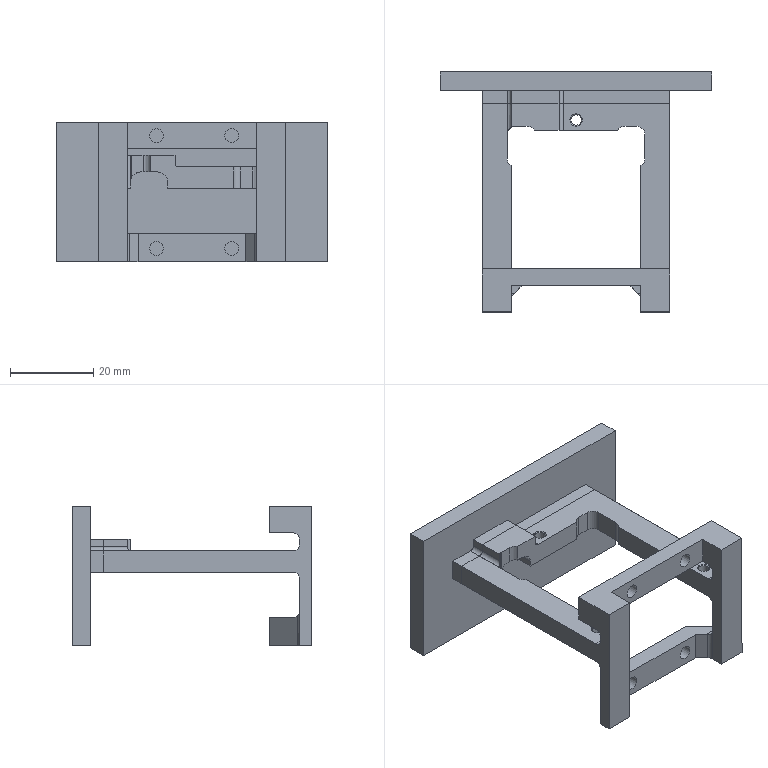NC program | NX | posted with a generic post | part box 65 x 57.5 x 33.5 mm
Lines 2192 to 2388 of 2388:
(DRILLING_1 , TOOL : 点孔D3-50-90度)
N4382 T12 M6
N4384 G54
N4386 G17 G0 G90 X8.5 Y18.03 S2000 M3
N4388 G43 Z26.75 H12
N4390 G94 G81 G98 Z-1.9 F150. R2.1
N4392 Y-17.97
N4394 X46. Y0.03
N4396 G80
N4398 G0 X46. Y0.03 Z26.75
N4400 M5
(DRILLING_1_COPY , TOOL : 钻头D2.5-35-61)
N4402 T10 M6
N4404 G54
N4406 G17 G0 G90 X8.5 Y18.03 S3000 M3
N4408 G43 Z26.75 H10
N4410 G94 G83 G98 Z-8.9 F150. Q2. R2.1
N4412 Y-17.97
N4414 X46. Y0.03
N4416 G80
N4418 G0 X46. Y0.03 Z26.75
N4420 M5
(DRILLING_1_COPY_COPY , TOOL : 上排M3-10-D4-52)
N4422 T11 M6
N4424 G54
N4426 G17 G0 G90 X8.5 Y18.03 S300 M3
N4428 G43 Z26.75 H11
N4430 G84 G94 G98 Z-7.9 F150. R2.1
N4432 Y-17.97
N4434 X46. Y0.03
N4436 G80
N4438 G0 X46. Y0.03 Z26.75
N4440 M5
(PLANAR_MILL_5 , TOOL : D3-9-D4-50-3T-FINISH)
N4442 T06 M6
N4444 G54
N4446 G17 G0 G90 X6.5 Y24.5 S3000 M3
N4448 G43 Z66.75 H6
N4450 Z10.3
N4452 G94 G1 Z8.3 F600.
N4454 G3 X4.5 Y22.5 R2.
N4456 G1 Y21.676
N4458 X11.361 Y14.816
N4460 G2 X11.8 Y13.755 R1.5
N4462 G1 Y-13.695
N4464 G2 X11.361 Y-14.756 R1.5
N4466 G1 X4.5 Y-21.616
N4468 Y-22.5
N4470 G3 X6.5 Y-24.5 R2.
N4472 G1 Z10.3
N4474 G0 Z66.75
N4476 Y24.5
N4478 Z10.3
N4480 G1 Z8.3
N4482 G3 X4.5 Y22.5 R2.
N4484 G1 Y21.676
N4486 X11.361 Y14.816
N4488 G2 X11.8 Y13.755 R1.5
N4490 G1 Y-13.695
N4492 G2 X11.361 Y-14.756 R1.5
N4494 G1 X4.5 Y-21.616
N4496 Y-22.5
N4498 G3 X6.5 Y-24.5 R2.
N4500 G1 Z10.3
N4502 G0 Z66.75
N4504 M5
(FLOOR_WALL_COPY_COPY , TOOL : D4-12-D4-50-3T-FINISH)
N4506 T04 M6
N4508 G54
N4510 G17 G0 G90 X38.5 Y5.986 S4000 M3
N4512 G43 Z70.5 H4
N4514 Z2.1
N4516 G94 G1 Z-0.9 F600.
N4518 X47.761
N4520 X47.5 Y2.997
N4522 Y-1.77
N4524 X48.
N4526 Y8.342
N4528 X47.5 Y10.278
N4530 Y17.5
N4532 G3 X45.5 Y19.5 R2.
N4534 G1 X35.
N4536 G3 X33.268 Y18.5 R2.
N4538 G1 X11.212
N4540 X10.212 Y19.5
N4542 X49.
N4544 Y10.074
N4546 G3 X47.5 Y10.278 R2.
N4548 G1 X48. Y8.342
N4550 G2 X47.5 Y7.764 R3.
N4552 G1 Y2.997
N4554 X44.5
N4556 Y-4.77
N4558 X51.
N4560 Y21.5
N4562 X6.288
N4564 Y20.595
N4566 X10.384 Y16.5
N4568 X34.423
N4570 X35. Y17.5
N4572 X45.5
N4574 Y10.
N4576 X44.5 Y9.423
N4578 Y2.997
N4580 Y1.997
N4582 X38.5
N4584 Z2.1
N4586 G0 Z70.5
(FLOOR_WALL_COPY_COPY_COPY , TOOL : D4-12-D4-50-3T-FINISH)
N4588 X29.435 Y-27.5
N4590 Z2.1
N4592 G1 Z-0.92
N4594 Y-19.7
N4596 X49.2
N4598 Y-17.57
N4600 X46.926
N4602 X46.902 Y-17.743
N4604 G2 X45.119 Y-19.3 R1.8
N4606 G1 X35.
N4608 G2 X33.441 Y-18.4 R1.8
N4610 G1 X33.383 Y-18.3
N4612 X11.069
N4614 X9.669 Y-19.7
N4616 X29.435
N4618 Y-21.5
N4620 X51.
N4622 Y-15.77
N4624 X45.355
N4626 X45.119 Y-17.5
N4628 X35.
N4630 X34.423 Y-16.5
N4632 X10.324
N4634 X6.288 Y-20.535
N4636 Y-21.5
N4638 X29.435
N4640 X30.435
N4642 Y-27.5
N4644 Z2.1
N4646 G0 Z70.5
N4648 M5
(PLANAR_MILL_6 , TOOL : 倒角D4-90度)
N4650 T08 M6
N4652 G54
N4654 G17 G0 G90 X12.792 Y0.943 S3500 M3
N4656 G43 Z66.75 H8
N4658 Z17.75
N4660 G94 G1 Z15.75 F1000.
N4662 G41 X12.3 Y1.03 D8
N4664 G3 X11.3 Y0.03 R1.
N4666 G1 Y-13.695
N4668 G2 X11.007 Y-14.402 R1.
N4670 G1 X4.146 Y-21.263
N4672 G3 X4. Y-21.616 R0.5
N4674 G1 Y-22.5
N4676 G2 X3. Y-23.5 R1.
N4678 G1 X0.
N4680 G2 X-1. Y-22.5 R1.
N4682 G1 Y-15.5
N4684 G2 X0. Y-14.5 R1.
N4686 G1 X3.093
N4688 G3 X3.446 Y-14.354 R0.5
N4690 G1 X5.3 Y-12.5
N4692 Y12.5
N4694 X3.446 Y14.354
N4696 G3 X3.093 Y14.5 R0.5
N4698 G1 X0.
N4700 G2 X-1. Y15.5 R1.
N4702 G1 Y22.5
N4704 G2 X0. Y23.5 R1.
N4706 G1 X3.
N4708 G2 X4. Y22.5 R1.
N4710 G1 Y21.676
N4712 G3 X4.146 Y21.323 R0.5
N4714 G1 X11.007 Y14.462
N4716 G2 X11.3 Y13.755 R1.
N4718 G1 Y0.03
N4720 G3 X12.3 Y-0.97 R1.
N4722 G40
N4724 G1 X12.792 Y-0.883
N4726 Z17.75
N4728 G0 Z66.75
N4730 M5
N4732 M2